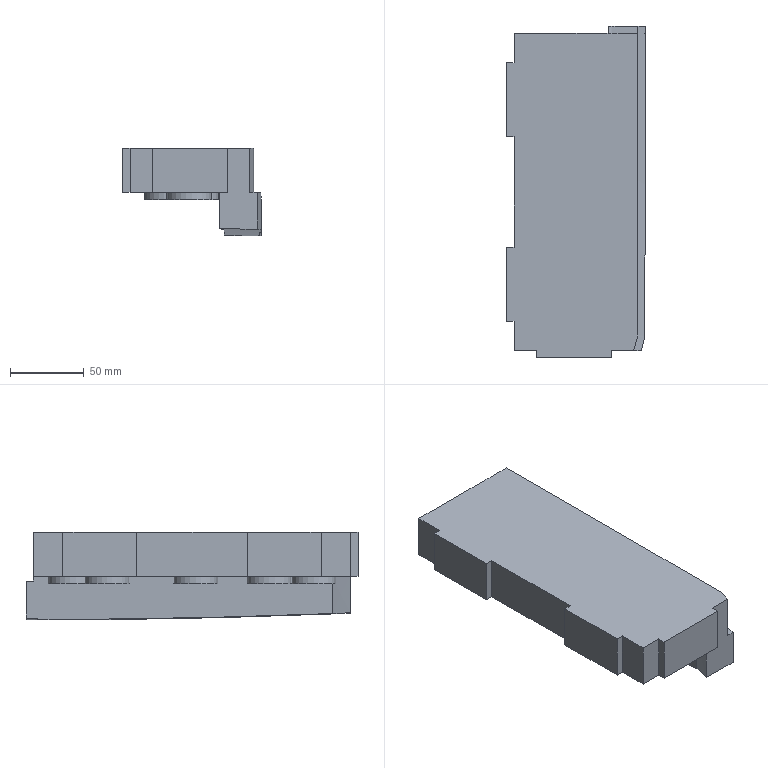Part | NX | features solid 2 | 1 solid | 38 faces | box 93.985 x 225 x 59.615 mm | volume 732225 mm3 | plane 22 | spline 11 | cylinder 5 | commonest cylinder face diameters 30 x5